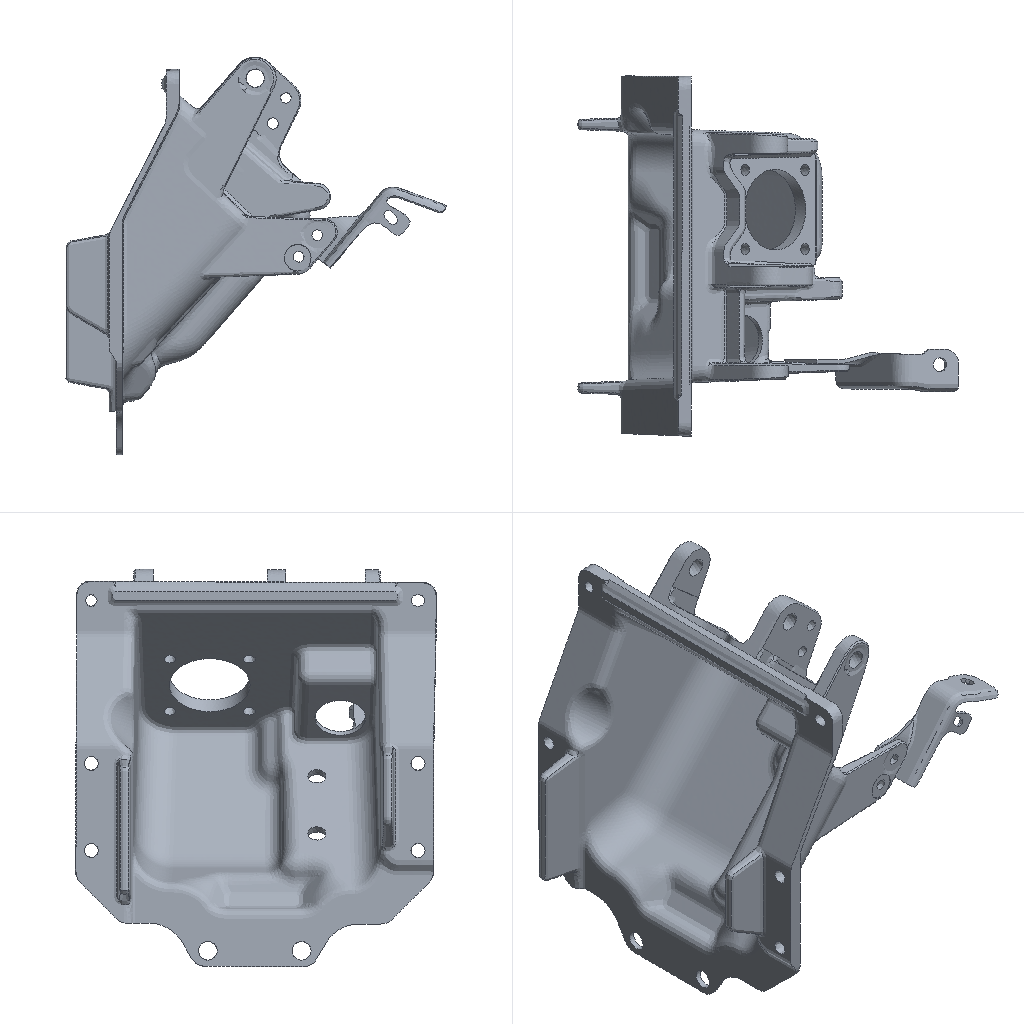Simulation study | nastran
Set-up summary:
category,name,step,type,value,unit,region
solver,nx_nastran
units,not stated in the deck,,not stated
analysis,deck,,modal,modal
analysis,solution,,SOL,103
load_step,SUBCASE 1,1,SUBCASE,SPC=2 LOAD=None
mesh,nodes,,,47580
mesh,elements,,,165540
element_type,CTETRA,,solid,165540
load,load commands in deck,,count,0
bc,support commands in deck,,count,8
check,setup vs results,,match,every grid point's frame and coordinates and every element id; grid points of CTETRA elements
Nastran input file, long lists of numbers shortened:
$$------------------------------------------------------------------------------$
$$                                                                              $
$$ NASTRAN Input Deck Generated by HyperMesh Version  :10.0buil                 $
$$ Generated using HyperMesh-Nastran Template Version : 10.0build60
$$                                                                              $
$$   Template:  general                                                         $
$$                                                                              $
$$------------------------------------------------------------------------------$
$$------------------------------------------------------------------------------$
$$                      Executive Control Cards                                 $
$$------------------------------------------------------------------------------$
SOL 103
CEND
$$------------------------------------------------------------------------------$
$$                      Case Control Cards                                      $
$$------------------------------------------------------------------------------$
  DISPLACEMENT = ALL
  ESE = ALL
$
$HMNAME LOADSTEP               1"modal"
SUBCASE       1
  LABEL=    modal
  SPC =        2
  METHOD(STRUCTURE) =        1
$$------------------------------------------------------------------------------$
$$                      Bulk Data Cards                                         $
$$------------------------------------------------------------------------------$
BEGIN BULK
PARAM,POST,-1
$$
$$  GRID Data
$$
GRID           1        -1112.7 -529.577646.4191
GRID           2        -1112.7 -531.536648.6338
$ (47578 more lines like these left out)
$$
$$  SPOINT Data
$$
$$
$$------------------------------------------------------------------------------$
$$             Group Definitions                                                $
$$------------------------------------------------------------------------------$
$$
$$ RBE2 Elements - Multiple dependent nodes
$$
RBE2      258993   52582  123456   41894   41895   41896   41897   41898+
+          41899   41900   41901   41922   41923   41924   41925   41926+
+          41927   41928   41929   41930   41931   41932   41933   41934+
+          41935   41936   41937   41938   41939   42338   42339   42340+
+          42341   42342   42343   42344   42345   42346   42347   42348+
+          42349   42350   42351   42352   42353   42354   42355   42356+
+          42357   43870
RBE2      258994   52583  123456   41436   41437   41438   41439   41440+
+          41441   41442   41443   41444   41445   41446   41447   41448+
+          41449   41450   41451   41452   41453   41454   41455   41456+
+          41457   41458   41459   41460   41461   41482   42122   42317+
+          42358   42359   42360   42361   42362   42363   42364   42365+
+          42366   42367   42368   42369   42370   42371   42372   42373+
+          42374   42375   42376   42377
$ (51 more lines like these left out)
$
$HMMOVE       18
$         258993THRU      259002
$
$$
$$------------------------------------------------------------------------------$
$$    HyperMesh name information for generic property collectors                $
$$------------------------------------------------------------------------------$
$$
$$------------------------------------------------------------------------------$
$$    Property Definition for 1-D Elements                                      $
$$------------------------------------------------------------------------------$
$
$  CTETRA elements 4-noded
$
CTETRA     89141       1   47228   44599   28642   28641
CTETRA     89142       1    9421    9457    9459   52560
$ (165538 more lines like these left out)
$
$HMMOVE       16
$          89141THRU      250583
$
$ (33 more lines like these left out)
PSOLID         1       1
$$
$$------------------------------------------------------------------------------$
$$                      Material Definition Cards                               $
$$------------------------------------------------------------------------------$
$$--------------------------------------------------------------
$$ HYPERMESH TAGS
$$--------------------------------------------------------------
$$BEGIN TAGS
$$END TAGS
$$
$$  MAT1 Data
$
$HMNAME MAT                    1"steel" "MAT1"
$HWCOLOR MAT                   1       3
MAT1           1210000.0        0.29    7.83E-09
$$
$$
$$
$$------------------------------------------------------------------------------$
$ (36 more lines like these left out)
EIGRL          11.0                    5                            MASS
$$
$$  SPC Data
$$
SPC            2   52588  1234560.0
SPC            2   52585  1234560.0
SPC            2   52589  1234560.0
SPC            2   52587  1234560.0
SPC            2   52586  1234560.0
SPC            2   52584  1234560.0
SPC            2   52591  1234560.0
SPC            2   52590  1234560.0
$
ENDDATA
Results summary:
result,analysis,,,modal
result,primary field,,,eigenvectors